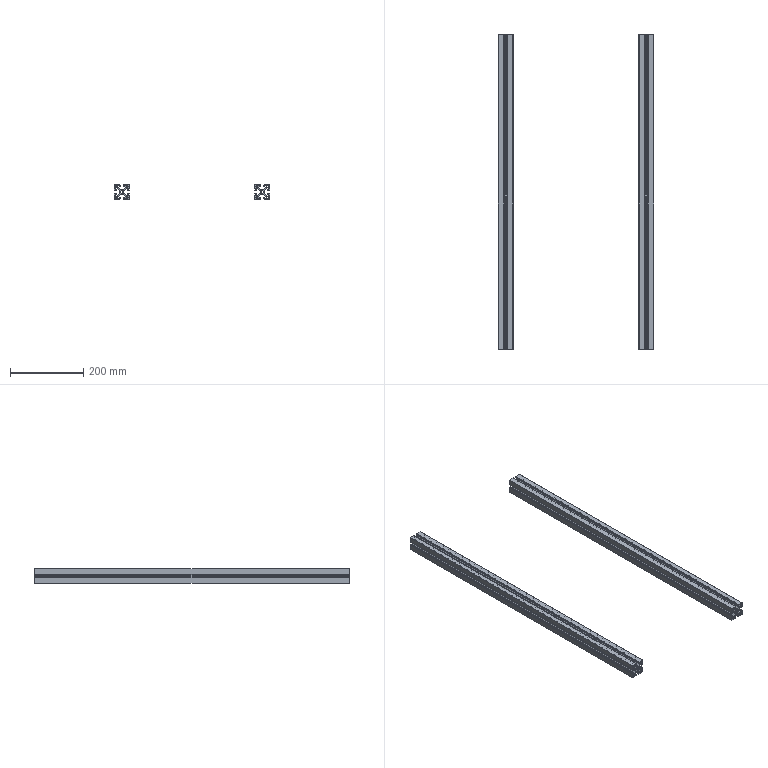Part | SolidWorks | features CoordSys 1, WeldMemberFeat 1, WeldmentFeature 1 | 2 solids | 346 faces | box 425 x 861 x 40 mm | volume 1154541 mm3 | cylinder 182 | plane 164 | commonest cylinder face diameters 1 x88 0.6 x58 4 x16 4.9 x16 6.8 x4